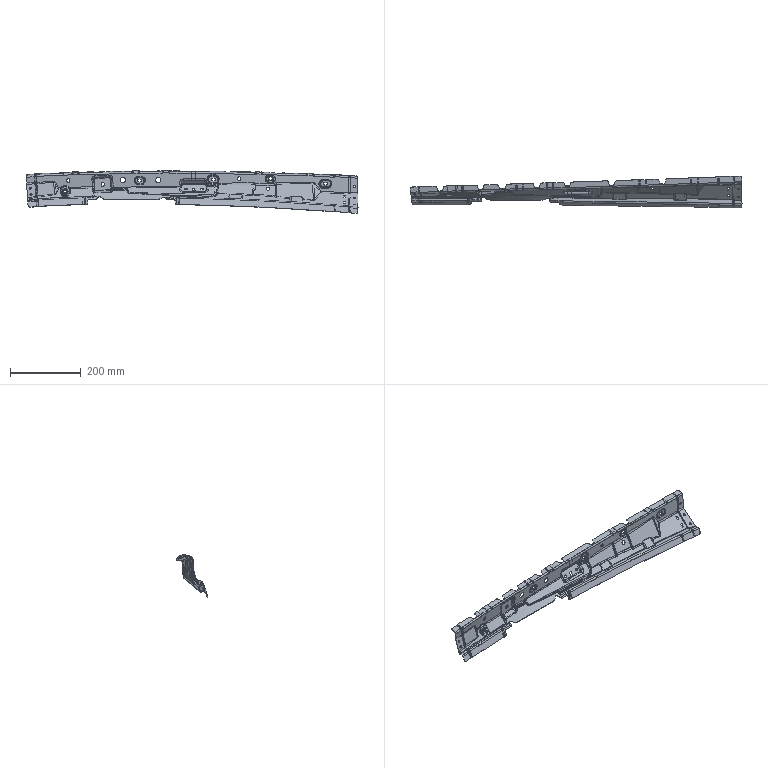Part | STEP file | FNA5401571 | 1 solid | 1420 faces | box 935.734 x 89.628 x 121.004 mm | volume 119563 mm3 | spline 1242 | cylinder 92 | plane 46 | other 28 | sphere 12 | commonest cylinder face diameters 6 x20 8 x17 7 x12 10 x9 12 x9 10.5 x8